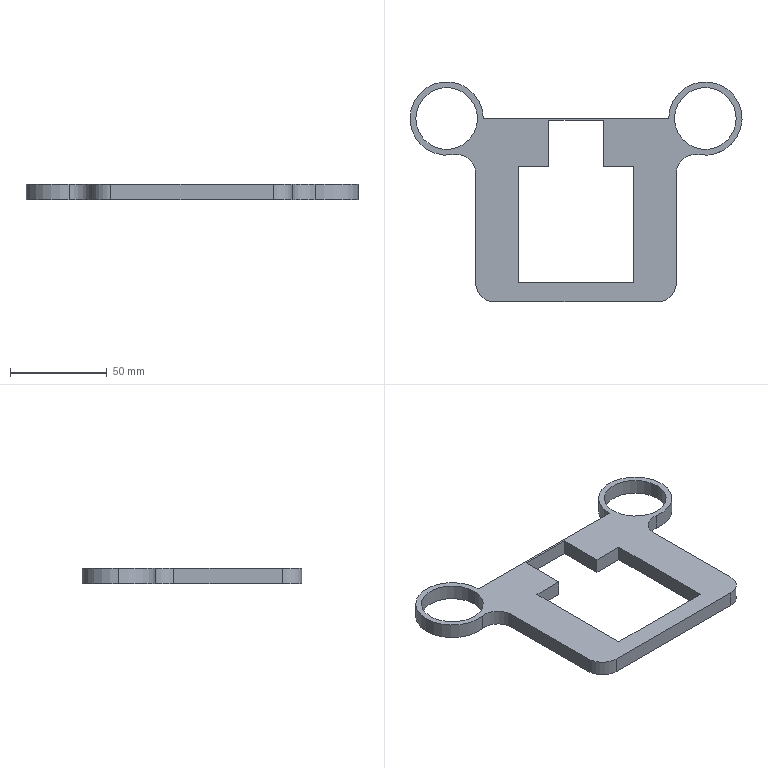Part | SolidWorks | features Extrusion 1 | 1 solid | 25 faces | box 172 x 114 x 8 mm | volume 50080 mm3 | plane 14 | cylinder 11 | commonest cylinder face diameters 20 x4 32 x4 38 x3
STEP:
#1=CARTESIAN_POINT('',(50.608,35.447,8.));
#2=VERTEX_POINT('',#1);
#3=CARTESIAN_POINT('',(82.608,35.447,8.));
#4=VERTEX_POINT('',#3);
#5=CARTESIAN_POINT('',(66.608,35.447,8.));
#6=DIRECTION('',(0.,0.,1.));
#7=DIRECTION('',(1.,0.,0.));
#8=AXIS2_PLACEMENT_3D('',#5,#6,#7);
#9=CIRCLE('',#8,16.);
#10=EDGE_CURVE('',#2,#4,#9,.T.);
#11=ORIENTED_EDGE('',*,*,#10,.T.);
#12=CARTESIAN_POINT('',(82.608,35.447,0.));
#13=VERTEX_POINT('',#12);
#14=CARTESIAN_POINT('',(82.608,35.447,8.));
#15=DIRECTION('',(0.,0.,-1.));
#16=VECTOR('',#15,1000.);
#17=LINE('',#14,#16);
#18=EDGE_CURVE('',#4,#13,#17,.T.);
#19=ORIENTED_EDGE('',*,*,#18,.T.);
#20=CARTESIAN_POINT('',(50.608,35.447,0.));
#21=VERTEX_POINT('',#20);
#22=CARTESIAN_POINT('',(66.608,35.447,0.));
#23=DIRECTION('',(0.,0.,1.));
#24=DIRECTION('',(1.,0.,0.));
#25=AXIS2_PLACEMENT_3D('',#22,#23,#24);
#26=CIRCLE('',#25,16.);
#27=EDGE_CURVE('',#21,#13,#26,.T.);
#28=ORIENTED_EDGE('',*,*,#27,.F.);
#29=CARTESIAN_POINT('',(50.608,35.447,8.));
#30=DIRECTION('',(0.,0.,-1.));
#31=VECTOR('',#30,1000.);
#32=LINE('',#29,#31);
#33=EDGE_CURVE('',#2,#21,#32,.T.);
#34=ORIENTED_EDGE('',*,*,#33,.F.);
#35=EDGE_LOOP('',(#11,#19,#28,#34));
#36=FACE_OUTER_BOUND('',#35,.T.);
#37=CARTESIAN_POINT('',(66.608,35.447,8.));
#38=DIRECTION('',(0.,0.,-1.));
#39=DIRECTION('',(-1.,0.,0.));
#40=AXIS2_PLACEMENT_3D('',#37,#38,#39);
#41=CYLINDRICAL_SURFACE('',#40,16.);
#42=ADVANCED_FACE('',(#36),#41,.F.);
#43=CARTESIAN_POINT('',(-83.392,35.447,8.));
#44=VERTEX_POINT('',#43);
#45=CARTESIAN_POINT('',(-51.392,35.447,8.));
#46=VERTEX_POINT('',#45);
#47=CARTESIAN_POINT('',(-67.392,35.447,8.));
#48=DIRECTION('',(0.,0.,1.));
#49=DIRECTION('',(1.,0.,0.));
#50=AXIS2_PLACEMENT_3D('',#47,#48,#49);
#51=CIRCLE('',#50,16.);
#52=EDGE_CURVE('',#44,#46,#51,.T.);
#53=ORIENTED_EDGE('',*,*,#52,.T.);
#54=CARTESIAN_POINT('',(-51.392,35.447,0.));
#55=VERTEX_POINT('',#54);
#56=CARTESIAN_POINT('',(-51.392,35.447,8.));
#57=DIRECTION('',(0.,0.,-1.));
#58=VECTOR('',#57,1000.);
#59=LINE('',#56,#58);
#60=EDGE_CURVE('',#46,#55,#59,.T.);
#61=ORIENTED_EDGE('',*,*,#60,.T.);
#62=CARTESIAN_POINT('',(-83.392,35.447,0.));
#63=VERTEX_POINT('',#62);
#64=CARTESIAN_POINT('',(-67.392,35.447,0.));
#65=DIRECTION('',(0.,0.,1.));
#66=DIRECTION('',(1.,0.,0.));
#67=AXIS2_PLACEMENT_3D('',#64,#65,#66);
#68=CIRCLE('',#67,16.);
#69=EDGE_CURVE('',#63,#55,#68,.T.);
#70=ORIENTED_EDGE('',*,*,#69,.F.);
#71=CARTESIAN_POINT('',(-83.392,35.447,8.));
#72=DIRECTION('',(0.,0.,-1.));
#73=VECTOR('',#72,1000.);
#74=LINE('',#71,#73);
#75=EDGE_CURVE('',#44,#63,#74,.T.);
#76=ORIENTED_EDGE('',*,*,#75,.F.);
#77=EDGE_LOOP('',(#53,#61,#70,#76));
#78=FACE_OUTER_BOUND('',#77,.T.);
#79=CARTESIAN_POINT('',(-67.392,35.447,8.));
#80=DIRECTION('',(0.,0.,-1.));
#81=DIRECTION('',(-1.,0.,0.));
#82=AXIS2_PLACEMENT_3D('',#79,#80,#81);
#83=CYLINDRICAL_SURFACE('',#82,16.);
#84=ADVANCED_FACE('',(#78),#83,.F.);
#85=CARTESIAN_POINT('',(-86.392,35.447,8.));
#86=VERTEX_POINT('',#85);
#87=CARTESIAN_POINT('',(-64.116,16.731,8.));
#88=VERTEX_POINT('',#87);
#89=CARTESIAN_POINT('',(-67.392,35.447,8.));
#90=DIRECTION('',(0.,0.,1.));
#91=DIRECTION('',(1.,0.,0.));
#92=AXIS2_PLACEMENT_3D('',#89,#90,#91);
#93=CIRCLE('',#92,19.);
#94=EDGE_CURVE('',#86,#88,#93,.T.);
#95=ORIENTED_EDGE('',*,*,#94,.F.);
#96=CARTESIAN_POINT('',(-86.392,35.447,0.));
#97=VERTEX_POINT('',#96);
#98=CARTESIAN_POINT('',(-86.392,35.447,8.));
#99=DIRECTION('',(0.,0.,-1.));
#100=VECTOR('',#99,1000.);
#101=LINE('',#98,#100);
#102=EDGE_CURVE('',#86,#97,#101,.T.);
#103=ORIENTED_EDGE('',*,*,#102,.T.);
#104=CARTESIAN_POINT('',(-64.116,16.731,0.));
#105=VERTEX_POINT('',#104);
#106=CARTESIAN_POINT('',(-67.392,35.447,0.));
#107=DIRECTION('',(0.,0.,1.));
#108=DIRECTION('',(1.,0.,0.));
#109=AXIS2_PLACEMENT_3D('',#106,#107,#108);
#110=CIRCLE('',#109,19.);
#111=EDGE_CURVE('',#97,#105,#110,.T.);
#112=ORIENTED_EDGE('',*,*,#111,.T.);
#113=CARTESIAN_POINT('',(-64.116,16.731,8.));
#114=DIRECTION('',(0.,0.,-1.));
#115=VECTOR('',#114,1000.);
#116=LINE('',#113,#115);
#117=EDGE_CURVE('',#88,#105,#116,.T.);
#118=ORIENTED_EDGE('',*,*,#117,.F.);
#119=EDGE_LOOP('',(#95,#103,#112,#118));
#120=FACE_OUTER_BOUND('',#119,.T.);
#121=CARTESIAN_POINT('',(-67.392,35.447,8.));
#122=DIRECTION('',(0.,0.,-1.));
#123=DIRECTION('',(-1.,0.,0.));
#124=AXIS2_PLACEMENT_3D('',#121,#122,#123);
#125=CYLINDRICAL_SURFACE('',#124,19.);
#126=ADVANCED_FACE('',(#120),#125,.T.);
#127=CARTESIAN_POINT('',(-14.392,34.447,0.));
#128=VERTEX_POINT('',#127);
#129=CARTESIAN_POINT('',(13.608,34.447,0.));
#130=VERTEX_POINT('',#129);
#131=CARTESIAN_POINT('',(0.,34.447,0.));
#132=DIRECTION('',(1.,0.,0.));
#133=VECTOR('',#132,1000.);
#134=LINE('',#131,#133);
#135=EDGE_CURVE('',#128,#130,#134,.T.);
#136=ORIENTED_EDGE('',*,*,#135,.T.);
#137=CARTESIAN_POINT('',(13.608,34.447,8.));
#138=VERTEX_POINT('',#137);
#139=CARTESIAN_POINT('',(13.608,34.447,8.));
#140=DIRECTION('',(0.,0.,-1.));
#141=VECTOR('',#140,1000.);
#142=LINE('',#139,#141);
#143=EDGE_CURVE('',#138,#130,#142,.T.);
#144=ORIENTED_EDGE('',*,*,#143,.F.);
#145=CARTESIAN_POINT('',(-14.392,34.447,8.));
#146=VERTEX_POINT('',#145);
#147=CARTESIAN_POINT('',(0.,34.447,8.));
#148=DIRECTION('',(1.,0.,0.));
#149=VECTOR('',#148,1000.);
#150=LINE('',#147,#149);
#151=EDGE_CURVE('',#146,#138,#150,.T.);
#152=ORIENTED_EDGE('',*,*,#151,.F.);
#153=CARTESIAN_POINT('',(-14.392,34.447,8.));
#154=DIRECTION('',(0.,0.,-1.));
#155=VECTOR('',#154,1000.);
#156=LINE('',#153,#155);
#157=EDGE_CURVE('',#146,#128,#156,.T.);
#158=ORIENTED_EDGE('',*,*,#157,.T.);
#159=EDGE_LOOP('',(#136,#144,#152,#158));
#160=FACE_OUTER_BOUND('',#159,.T.);
#161=CARTESIAN_POINT('',(0.,34.447,8.));
#162=DIRECTION('',(0.,1.,0.));
#163=DIRECTION('',(-1.,0.,0.));
#164=AXIS2_PLACEMENT_3D('',#161,#162,#163);
#165=PLANE('',#164);
#166=ADVANCED_FACE('',(#160),#165,.F.);
#167=CARTESIAN_POINT('',(13.608,10.447,0.));
#168=VERTEX_POINT('',#167);
#169=CARTESIAN_POINT('',(13.608,0.,0.));
#170=DIRECTION('',(0.,-1.,0.));
#171=VECTOR('',#170,1000.);
#172=LINE('',#169,#171);
#173=EDGE_CURVE('',#130,#168,#172,.T.);
#174=ORIENTED_EDGE('',*,*,#173,.T.);
#175=CARTESIAN_POINT('',(13.608,10.447,8.));
#176=VERTEX_POINT('',#175);
#177=CARTESIAN_POINT('',(13.608,10.447,8.));
#178=DIRECTION('',(0.,0.,-1.));
#179=VECTOR('',#178,1000.);
#180=LINE('',#177,#179);
#181=EDGE_CURVE('',#176,#168,#180,.T.);
#182=ORIENTED_EDGE('',*,*,#181,.F.);
#183=CARTESIAN_POINT('',(13.608,0.,8.));
#184=DIRECTION('',(0.,-1.,0.));
#185=VECTOR('',#184,1000.);
#186=LINE('',#183,#185);
#187=EDGE_CURVE('',#138,#176,#186,.T.);
#188=ORIENTED_EDGE('',*,*,#187,.F.);
#189=ORIENTED_EDGE('',*,*,#143,.T.);
#190=EDGE_LOOP('',(#174,#182,#188,#189));
#191=FACE_OUTER_BOUND('',#190,.T.);
#192=CARTESIAN_POINT('',(13.608,0.,8.));
#193=DIRECTION('',(1.,0.,0.));
#194=DIRECTION('',(0.,1.,0.));
#195=AXIS2_PLACEMENT_3D('',#192,#193,#194);
#196=PLANE('',#195);
#197=ADVANCED_FACE('',(#191),#196,.F.);
#198=CARTESIAN_POINT('',(29.608,10.447,0.));
#199=VERTEX_POINT('',#198);
#200=CARTESIAN_POINT('',(0.,10.447,0.));
#201=DIRECTION('',(1.,0.,0.));
#202=VECTOR('',#201,1000.);
#203=LINE('',#200,#202);
#204=EDGE_CURVE('',#168,#199,#203,.T.);
#205=ORIENTED_EDGE('',*,*,#204,.T.);
#206=CARTESIAN_POINT('',(29.608,10.447,8.));
#207=VERTEX_POINT('',#206);
#208=CARTESIAN_POINT('',(29.608,10.447,8.));
#209=DIRECTION('',(0.,0.,-1.));
#210=VECTOR('',#209,1000.);
#211=LINE('',#208,#210);
#212=EDGE_CURVE('',#207,#199,#211,.T.);
#213=ORIENTED_EDGE('',*,*,#212,.F.);
#214=CARTESIAN_POINT('',(0.,10.447,8.));
#215=DIRECTION('',(1.,0.,0.));
#216=VECTOR('',#215,1000.);
#217=LINE('',#214,#216);
#218=EDGE_CURVE('',#176,#207,#217,.T.);
#219=ORIENTED_EDGE('',*,*,#218,.F.);
#220=ORIENTED_EDGE('',*,*,#181,.T.);
#221=EDGE_LOOP('',(#205,#213,#219,#220));
#222=FACE_OUTER_BOUND('',#221,.T.);
#223=CARTESIAN_POINT('',(0.,10.447,8.));
#224=DIRECTION('',(0.,1.,0.));
#225=DIRECTION('',(0.,0.,1.));
#226=AXIS2_PLACEMENT_3D('',#223,#224,#225);
#227=PLANE('',#226);
#228=ADVANCED_FACE('',(#222),#227,.F.);
#229=CARTESIAN_POINT('',(29.608,-49.553,0.));
#230=VERTEX_POINT('',#229);
#231=CARTESIAN_POINT('',(29.608,0.,0.));
#232=DIRECTION('',(0.,-1.,0.));
#233=VECTOR('',#232,1000.);
#234=LINE('',#231,#233);
#235=EDGE_CURVE('',#199,#230,#234,.T.);
#236=ORIENTED_EDGE('',*,*,#235,.T.);
#237=CARTESIAN_POINT('',(29.608,-49.553,8.));
#238=VERTEX_POINT('',#237);
#239=CARTESIAN_POINT('',(29.608,-49.553,8.));
#240=DIRECTION('',(0.,0.,-1.));
#241=VECTOR('',#240,1000.);
#242=LINE('',#239,#241);
#243=EDGE_CURVE('',#238,#230,#242,.T.);
#244=ORIENTED_EDGE('',*,*,#243,.F.);
#245=CARTESIAN_POINT('',(29.608,0.,8.));
#246=DIRECTION('',(0.,-1.,0.));
#247=VECTOR('',#246,1000.);
#248=LINE('',#245,#247);
#249=EDGE_CURVE('',#207,#238,#248,.T.);
#250=ORIENTED_EDGE('',*,*,#249,.F.);
#251=ORIENTED_EDGE('',*,*,#212,.T.);
#252=EDGE_LOOP('',(#236,#244,#250,#251));
#253=FACE_OUTER_BOUND('',#252,.T.);
#254=CARTESIAN_POINT('',(29.608,0.,8.));
#255=DIRECTION('',(1.,0.,0.));
#256=DIRECTION('',(0.,1.,0.));
#257=AXIS2_PLACEMENT_3D('',#254,#255,#256);
#258=PLANE('',#257);
#259=ADVANCED_FACE('',(#253),#258,.F.);
#260=CARTESIAN_POINT('',(-30.392,-49.553,0.));
#261=VERTEX_POINT('',#260);
#262=CARTESIAN_POINT('',(0.,-49.553,0.));
#263=DIRECTION('',(-1.,0.,0.));
#264=VECTOR('',#263,1000.);
#265=LINE('',#262,#264);
#266=EDGE_CURVE('',#230,#261,#265,.T.);
#267=ORIENTED_EDGE('',*,*,#266,.T.);
#268=CARTESIAN_POINT('',(-30.392,-49.553,8.));
#269=VERTEX_POINT('',#268);
#270=CARTESIAN_POINT('',(-30.392,-49.553,8.));
#271=DIRECTION('',(0.,0.,-1.));
#272=VECTOR('',#271,1000.);
#273=LINE('',#270,#272);
#274=EDGE_CURVE('',#269,#261,#273,.T.);
#275=ORIENTED_EDGE('',*,*,#274,.F.);
#276=CARTESIAN_POINT('',(0.,-49.553,8.));
#277=DIRECTION('',(-1.,0.,0.));
#278=VECTOR('',#277,1000.);
#279=LINE('',#276,#278);
#280=EDGE_CURVE('',#238,#269,#279,.T.);
#281=ORIENTED_EDGE('',*,*,#280,.F.);
#282=ORIENTED_EDGE('',*,*,#243,.T.);
#283=EDGE_LOOP('',(#267,#275,#281,#282));
#284=FACE_OUTER_BOUND('',#283,.T.);
#285=CARTESIAN_POINT('',(0.,-49.553,8.));
#286=DIRECTION('',(0.,-1.,0.));
#287=DIRECTION('',(0.,0.,-1.));
#288=AXIS2_PLACEMENT_3D('',#285,#286,#287);
#289=PLANE('',#288);
#290=ADVANCED_FACE('',(#284),#289,.F.);
#291=CARTESIAN_POINT('',(-30.392,10.447,0.));
#292=VERTEX_POINT('',#291);
#293=CARTESIAN_POINT('',(-30.392,0.,0.));
#294=DIRECTION('',(0.,1.,0.));
#295=VECTOR('',#294,1000.);
#296=LINE('',#293,#295);
#297=EDGE_CURVE('',#261,#292,#296,.T.);
#298=ORIENTED_EDGE('',*,*,#297,.T.);
#299=CARTESIAN_POINT('',(-30.392,10.447,8.));
#300=VERTEX_POINT('',#299);
#301=CARTESIAN_POINT('',(-30.392,10.447,8.));
#302=DIRECTION('',(0.,0.,-1.));
#303=VECTOR('',#302,1000.);
#304=LINE('',#301,#303);
#305=EDGE_CURVE('',#300,#292,#304,.T.);
#306=ORIENTED_EDGE('',*,*,#305,.F.);
#307=CARTESIAN_POINT('',(-30.392,0.,8.));
#308=DIRECTION('',(0.,1.,0.));
#309=VECTOR('',#308,1000.);
#310=LINE('',#307,#309);
#311=EDGE_CURVE('',#269,#300,#310,.T.);
#312=ORIENTED_EDGE('',*,*,#311,.F.);
#313=ORIENTED_EDGE('',*,*,#274,.T.);
#314=EDGE_LOOP('',(#298,#306,#312,#313));
#315=FACE_OUTER_BOUND('',#314,.T.);
#316=CARTESIAN_POINT('',(-30.392,0.,8.));
#317=DIRECTION('',(-1.,0.,0.));
#318=DIRECTION('',(0.,-1.,0.));
#319=AXIS2_PLACEMENT_3D('',#316,#317,#318);
#320=PLANE('',#319);
#321=ADVANCED_FACE('',(#315),#320,.F.);
#322=CARTESIAN_POINT('',(-14.392,10.447,0.));
#323=VERTEX_POINT('',#322);
#324=CARTESIAN_POINT('',(0.,10.447,0.));
#325=DIRECTION('',(1.,0.,0.));
#326=VECTOR('',#325,1000.);
#327=LINE('',#324,#326);
#328=EDGE_CURVE('',#292,#323,#327,.T.);
#329=ORIENTED_EDGE('',*,*,#328,.T.);
#330=CARTESIAN_POINT('',(-14.392,10.447,8.));
#331=VERTEX_POINT('',#330);
#332=CARTESIAN_POINT('',(-14.392,10.447,8.));
#333=DIRECTION('',(0.,0.,-1.));
#334=VECTOR('',#333,1000.);
#335=LINE('',#332,#334);
#336=EDGE_CURVE('',#331,#323,#335,.T.);
#337=ORIENTED_EDGE('',*,*,#336,.F.);
#338=CARTESIAN_POINT('',(0.,10.447,8.));
#339=DIRECTION('',(1.,0.,0.));
#340=VECTOR('',#339,1000.);
#341=LINE('',#338,#340);
#342=EDGE_CURVE('',#300,#331,#341,.T.);
#343=ORIENTED_EDGE('',*,*,#342,.F.);
#344=ORIENTED_EDGE('',*,*,#305,.T.);
#345=EDGE_LOOP('',(#329,#337,#343,#344));
#346=FACE_OUTER_BOUND('',#345,.T.);
#347=CARTESIAN_POINT('',(0.,10.447,8.));
#348=DIRECTION('',(0.,1.,0.));
#349=DIRECTION('',(0.,0.,1.));
#350=AXIS2_PLACEMENT_3D('',#347,#348,#349);
#351=PLANE('',#350);
#352=ADVANCED_FACE('',(#346),#351,.F.);
#353=CARTESIAN_POINT('',(63.332,16.731,0.));
#354=VERTEX_POINT('',#353);
#355=CARTESIAN_POINT('',(47.608,35.447,0.));
#356=VERTEX_POINT('',#355);
#357=CARTESIAN_POINT('',(66.608,35.447,0.));
#358=DIRECTION('',(0.,0.,1.));
#359=DIRECTION('',(1.,0.,0.));
#360=AXIS2_PLACEMENT_3D('',#357,#358,#359);
#361=CIRCLE('',#360,19.);
#362=EDGE_CURVE('',#354,#356,#361,.T.);
#363=ORIENTED_EDGE('',*,*,#362,.T.);
#364=CARTESIAN_POINT('',(47.608,35.447,8.));
#365=VERTEX_POINT('',#364);
#366=CARTESIAN_POINT('',(47.608,35.447,8.));
#367=DIRECTION('',(0.,0.,-1.));
#368=VECTOR('',#367,1000.);
#369=LINE('',#366,#368);
#370=EDGE_CURVE('',#365,#356,#369,.T.);
#371=ORIENTED_EDGE('',*,*,#370,.F.);
#372=CARTESIAN_POINT('',(63.332,16.731,8.));
#373=VERTEX_POINT('',#372);
#374=CARTESIAN_POINT('',(66.608,35.447,8.));
#375=DIRECTION('',(0.,0.,1.));
#376=DIRECTION('',(1.,0.,0.));
#377=AXIS2_PLACEMENT_3D('',#374,#375,#376);
#378=CIRCLE('',#377,19.);
#379=EDGE_CURVE('',#373,#365,#378,.T.);
#380=ORIENTED_EDGE('',*,*,#379,.F.);
#381=CARTESIAN_POINT('',(63.332,16.731,8.));
#382=DIRECTION('',(0.,0.,-1.));
#383=VECTOR('',#382,1000.);
#384=LINE('',#381,#383);
#385=EDGE_CURVE('',#373,#354,#384,.T.);
#386=ORIENTED_EDGE('',*,*,#385,.T.);
#387=EDGE_LOOP('',(#363,#371,#380,#386));
#388=FACE_OUTER_BOUND('',#387,.T.);
#389=CARTESIAN_POINT('',(66.608,35.447,8.));
#390=DIRECTION('',(0.,0.,-1.));
#391=DIRECTION('',(-1.,0.,0.));
#392=AXIS2_PLACEMENT_3D('',#389,#390,#391);
#393=CYLINDRICAL_SURFACE('',#392,19.);
#394=ADVANCED_FACE('',(#388),#393,.T.);
#395=CARTESIAN_POINT('',(-48.392,35.447,0.));
#396=VERTEX_POINT('',#395);
#397=CARTESIAN_POINT('',(0.,35.447,0.));
#398=DIRECTION('',(-1.,0.,0.));
#399=VECTOR('',#398,1000.);
#400=LINE('',#397,#399);
#401=EDGE_CURVE('',#356,#396,#400,.T.);
#402=ORIENTED_EDGE('',*,*,#401,.T.);
#403=CARTESIAN_POINT('',(-48.392,35.447,8.));
#404=VERTEX_POINT('',#403);
#405=CARTESIAN_POINT('',(-48.392,35.447,8.));
#406=DIRECTION('',(0.,0.,-1.));
#407=VECTOR('',#406,1000.);
#408=LINE('',#405,#407);
#409=EDGE_CURVE('',#404,#396,#408,.T.);
#410=ORIENTED_EDGE('',*,*,#409,.F.);
#411=CARTESIAN_POINT('',(0.,35.447,8.));
#412=DIRECTION('',(-1.,0.,0.));
#413=VECTOR('',#412,1000.);
#414=LINE('',#411,#413);
#415=EDGE_CURVE('',#365,#404,#414,.T.);
#416=ORIENTED_EDGE('',*,*,#415,.F.);
#417=ORIENTED_EDGE('',*,*,#370,.T.);
#418=EDGE_LOOP('',(#402,#410,#416,#417));
#419=FACE_OUTER_BOUND('',#418,.T.);
#420=CARTESIAN_POINT('',(0.,35.447,8.));
#421=DIRECTION('',(0.,-1.,0.));
#422=DIRECTION('',(0.,0.,-1.));
#423=AXIS2_PLACEMENT_3D('',#420,#421,#422);
#424=PLANE('',#423);
#425=ADVANCED_FACE('',(#419),#424,.F.);
#426=ORIENTED_EDGE('',*,*,#102,.F.);
#427=CARTESIAN_POINT('',(-67.392,35.447,8.));
#428=DIRECTION('',(0.,0.,1.));
#429=DIRECTION('',(1.,0.,0.));
#430=AXIS2_PLACEMENT_3D('',#427,#428,#429);
#431=CIRCLE('',#430,19.);
#432=EDGE_CURVE('',#404,#86,#431,.T.);
#433=ORIENTED_EDGE('',*,*,#432,.F.);
#434=ORIENTED_EDGE('',*,*,#409,.T.);
#435=CARTESIAN_POINT('',(-67.392,35.447,0.));
#436=DIRECTION('',(0.,0.,1.));
#437=DIRECTION('',(1.,0.,0.));
#438=AXIS2_PLACEMENT_3D('',#435,#436,#437);
#439=CIRCLE('',#438,19.);
#440=EDGE_CURVE('',#396,#97,#439,.T.);
#441=ORIENTED_EDGE('',*,*,#440,.T.);
#442=EDGE_LOOP('',(#426,#433,#434,#441));
#443=FACE_OUTER_BOUND('',#442,.T.);
#444=CARTESIAN_POINT('',(-67.392,35.447,8.));
#445=DIRECTION('',(0.,0.,-1.));
#446=DIRECTION('',(-1.,0.,0.));
#447=AXIS2_PLACEMENT_3D('',#444,#445,#446);
#448=CYLINDRICAL_SURFACE('',#447,19.);
#449=ADVANCED_FACE('',(#443),#448,.T.);
#450=CARTESIAN_POINT('',(-52.392,6.881,0.));
#451=VERTEX_POINT('',#450);
#452=CARTESIAN_POINT('',(-62.392,6.881,0.));
#453=DIRECTION('',(0.,0.,1.));
#454=DIRECTION('',(1.,0.,0.));
#455=AXIS2_PLACEMENT_3D('',#452,#453,#454);
#456=CIRCLE('',#455,10.);
#457=EDGE_CURVE('',#451,#105,#456,.T.);
#458=ORIENTED_EDGE('',*,*,#457,.F.);
#459=CARTESIAN_POINT('',(-52.392,6.881,8.));
#460=VERTEX_POINT('',#459);
#461=CARTESIAN_POINT('',(-52.392,6.881,8.));
#462=DIRECTION('',(0.,0.,-1.));
#463=VECTOR('',#462,1000.);
#464=LINE('',#461,#463);
#465=EDGE_CURVE('',#460,#451,#464,.T.);
#466=ORIENTED_EDGE('',*,*,#465,.F.);
#467=CARTESIAN_POINT('',(-62.392,6.881,8.));
#468=DIRECTION('',(0.,0.,1.));
#469=DIRECTION('',(1.,0.,0.));
#470=AXIS2_PLACEMENT_3D('',#467,#468,#469);
#471=CIRCLE('',#470,10.);
#472=EDGE_CURVE('',#460,#88,#471,.T.);
#473=ORIENTED_EDGE('',*,*,#472,.T.);
#474=ORIENTED_EDGE('',*,*,#117,.T.);
#475=EDGE_LOOP('',(#458,#466,#473,#474));
#476=FACE_OUTER_BOUND('',#475,.T.);
#477=CARTESIAN_POINT('',(-62.392,6.881,8.));
#478=DIRECTION('',(0.,0.,-1.));
#479=DIRECTION('',(-1.,0.,0.));
#480=AXIS2_PLACEMENT_3D('',#477,#478,#479);
#481=CYLINDRICAL_SURFACE('',#480,10.);
#482=ADVANCED_FACE('',(#476),#481,.F.);
#483=CARTESIAN_POINT('',(-52.392,-49.553,0.));
#484=VERTEX_POINT('',#483);
#485=CARTESIAN_POINT('',(-52.392,0.,0.));
#486=DIRECTION('',(0.,-1.,0.));
#487=VECTOR('',#486,1000.);
#488=LINE('',#485,#487);
#489=EDGE_CURVE('',#451,#484,#488,.T.);
#490=ORIENTED_EDGE('',*,*,#489,.T.);
#491=CARTESIAN_POINT('',(-52.392,-49.553,8.));
#492=VERTEX_POINT('',#491);
#493=CARTESIAN_POINT('',(-52.392,-49.553,8.));
#494=DIRECTION('',(0.,0.,-1.));
#495=VECTOR('',#494,1000.);
#496=LINE('',#493,#495);
#497=EDGE_CURVE('',#492,#484,#496,.T.);
#498=ORIENTED_EDGE('',*,*,#497,.F.);
#499=CARTESIAN_POINT('',(-52.392,0.,8.));
#500=DIRECTION('',(0.,-1.,0.));
#501=VECTOR('',#500,1000.);
#502=LINE('',#499,#501);
#503=EDGE_CURVE('',#460,#492,#502,.T.);
#504=ORIENTED_EDGE('',*,*,#503,.F.);
#505=ORIENTED_EDGE('',*,*,#465,.T.);
#506=EDGE_LOOP('',(#490,#498,#504,#505));
#507=FACE_OUTER_BOUND('',#506,.T.);
#508=CARTESIAN_POINT('',(-52.392,0.,8.));
#509=DIRECTION('',(1.,0.,0.));
#510=DIRECTION('',(0.,1.,0.));
#511=AXIS2_PLACEMENT_3D('',#508,#509,#510);
#512=PLANE('',#511);
#513=ADVANCED_FACE('',(#507),#512,.F.);
#514=CARTESIAN_POINT('',(-42.392,-59.553,0.));
#515=VERTEX_POINT('',#514);
#516=CARTESIAN_POINT('',(-42.392,-49.553,0.));
#517=DIRECTION('',(0.,0.,1.));
#518=DIRECTION('',(1.,0.,0.));
#519=AXIS2_PLACEMENT_3D('',#516,#517,#518);
#520=CIRCLE('',#519,10.);
#521=EDGE_CURVE('',#484,#515,#520,.T.);
#522=ORIENTED_EDGE('',*,*,#521,.T.);
#523=CARTESIAN_POINT('',(-42.392,-59.553,8.));
#524=VERTEX_POINT('',#523);
#525=CARTESIAN_POINT('',(-42.392,-59.553,8.));
#526=DIRECTION('',(0.,0.,-1.));
#527=VECTOR('',#526,1000.);
#528=LINE('',#525,#527);
#529=EDGE_CURVE('',#524,#515,#528,.T.);
#530=ORIENTED_EDGE('',*,*,#529,.F.);
#531=CARTESIAN_POINT('',(-42.392,-49.553,8.));
#532=DIRECTION('',(0.,0.,1.));
#533=DIRECTION('',(1.,0.,0.));
#534=AXIS2_PLACEMENT_3D('',#531,#532,#533);
#535=CIRCLE('',#534,10.);
#536=EDGE_CURVE('',#492,#524,#535,.T.);
#537=ORIENTED_EDGE('',*,*,#536,.F.);
#538=ORIENTED_EDGE('',*,*,#497,.T.);
#539=EDGE_LOOP('',(#522,#530,#537,#538));
#540=FACE_OUTER_BOUND('',#539,.T.);
#541=CARTESIAN_POINT('',(-42.392,-49.553,8.));
#542=DIRECTION('',(0.,0.,-1.));
#543=DIRECTION('',(-1.,0.,0.));
#544=AXIS2_PLACEMENT_3D('',#541,#542,#543);
#545=CYLINDRICAL_SURFACE('',#544,10.);
#546=ADVANCED_FACE('',(#540),#545,.T.);
#547=CARTESIAN_POINT('',(41.608,-59.553,0.));
#548=VERTEX_POINT('',#547);
#549=CARTESIAN_POINT('',(0.,-59.553,0.));
#550=DIRECTION('',(1.,0.,0.));
#551=VECTOR('',#550,1000.);
#552=LINE('',#549,#551);
#553=EDGE_CURVE('',#515,#548,#552,.T.);
#554=ORIENTED_EDGE('',*,*,#553,.T.);
#555=CARTESIAN_POINT('',(41.608,-59.553,8.));
#556=VERTEX_POINT('',#555);
#557=CARTESIAN_POINT('',(41.608,-59.553,8.));
#558=DIRECTION('',(0.,0.,-1.));
#559=VECTOR('',#558,1000.);
#560=LINE('',#557,#559);
#561=EDGE_CURVE('',#556,#548,#560,.T.);
#562=ORIENTED_EDGE('',*,*,#561,.F.);
#563=CARTESIAN_POINT('',(0.,-59.553,8.));
#564=DIRECTION('',(1.,0.,0.));
#565=VECTOR('',#564,1000.);
#566=LINE('',#563,#565);
#567=EDGE_CURVE('',#524,#556,#566,.T.);
#568=ORIENTED_EDGE('',*,*,#567,.F.);
#569=ORIENTED_EDGE('',*,*,#529,.T.);
#570=EDGE_LOOP('',(#554,#562,#568,#569));
#571=FACE_OUTER_BOUND('',#570,.T.);
#572=CARTESIAN_POINT('',(0.,-59.553,8.));
#573=DIRECTION('',(0.,1.,0.));
#574=DIRECTION('',(0.,0.,1.));
#575=AXIS2_PLACEMENT_3D('',#572,#573,#574);
#576=PLANE('',#575);
#577=ADVANCED_FACE('',(#571),#576,.F.);
#578=CARTESIAN_POINT('',(51.608,-49.553,0.));
#579=VERTEX_POINT('',#578);
#580=CARTESIAN_POINT('',(41.608,-49.553,0.));
#581=DIRECTION('',(0.,0.,-1.));
#582=DIRECTION('',(1.,0.,0.));
#583=AXIS2_PLACEMENT_3D('',#580,#581,#582);
#584=CIRCLE('',#583,10.);
#585=EDGE_CURVE('',#579,#548,#584,.T.);
#586=ORIENTED_EDGE('',*,*,#585,.F.);
#587=CARTESIAN_POINT('',(51.608,-49.553,8.));
#588=VERTEX_POINT('',#587);
#589=CARTESIAN_POINT('',(51.608,-49.553,8.));
#590=DIRECTION('',(0.,0.,-1.));
#591=VECTOR('',#590,1000.);
#592=LINE('',#589,#591);
#593=EDGE_CURVE('',#588,#579,#592,.T.);
#594=ORIENTED_EDGE('',*,*,#593,.F.);
#595=CARTESIAN_POINT('',(41.608,-49.553,8.));
#596=DIRECTION('',(0.,0.,-1.));
#597=DIRECTION('',(1.,0.,0.));
#598=AXIS2_PLACEMENT_3D('',#595,#596,#597);
#599=CIRCLE('',#598,10.);
#600=EDGE_CURVE('',#588,#556,#599,.T.);
#601=ORIENTED_EDGE('',*,*,#600,.T.);
#602=ORIENTED_EDGE('',*,*,#561,.T.);
#603=EDGE_LOOP('',(#586,#594,#601,#602));
#604=FACE_OUTER_BOUND('',#603,.T.);
#605=CARTESIAN_POINT('',(41.608,-49.553,8.));
#606=DIRECTION('',(0.,0.,-1.));
#607=DIRECTION('',(-1.,0.,0.));
#608=AXIS2_PLACEMENT_3D('',#605,#606,#607);
#609=CYLINDRICAL_SURFACE('',#608,10.);
#610=ADVANCED_FACE('',(#604),#609,.T.);
#611=CARTESIAN_POINT('',(51.608,6.881,0.));
#612=VERTEX_POINT('',#611);
#613=CARTESIAN_POINT('',(51.608,0.,0.));
#614=DIRECTION('',(0.,-1.,0.));
#615=VECTOR('',#614,1000.);
#616=LINE('',#613,#615);
#617=EDGE_CURVE('',#612,#579,#616,.T.);
#618=ORIENTED_EDGE('',*,*,#617,.F.);
#619=CARTESIAN_POINT('',(51.608,6.881,8.));
#620=VERTEX_POINT('',#619);
#621=CARTESIAN_POINT('',(51.608,6.881,8.));
#622=DIRECTION('',(0.,0.,-1.));
#623=VECTOR('',#622,1000.);
#624=LINE('',#621,#623);
#625=EDGE_CURVE('',#620,#612,#624,.T.);
#626=ORIENTED_EDGE('',*,*,#625,.F.);
#627=CARTESIAN_POINT('',(51.608,0.,8.));
#628=DIRECTION('',(0.,-1.,0.));
#629=VECTOR('',#628,1000.);
#630=LINE('',#627,#629);
#631=EDGE_CURVE('',#620,#588,#630,.T.);
#632=ORIENTED_EDGE('',*,*,#631,.T.);
#633=ORIENTED_EDGE('',*,*,#593,.T.);
#634=EDGE_LOOP('',(#618,#626,#632,#633));
#635=FACE_OUTER_BOUND('',#634,.T.);
#636=CARTESIAN_POINT('',(51.608,0.,8.));
#637=DIRECTION('',(1.,0.,0.));
#638=DIRECTION('',(0.,1.,0.));
#639=AXIS2_PLACEMENT_3D('',#636,#637,#638);
#640=PLANE('',#639);
#641=ADVANCED_FACE('',(#635),#640,.T.);
#642=ORIENTED_EDGE('',*,*,#60,.F.);
#643=CARTESIAN_POINT('',(-67.392,35.447,8.));
#644=DIRECTION('',(0.,0.,1.));
#645=DIRECTION('',(1.,0.,0.));
#646=AXIS2_PLACEMENT_3D('',#643,#644,#645);
#647=CIRCLE('',#646,16.);
#648=EDGE_CURVE('',#46,#44,#647,.T.);
#649=ORIENTED_EDGE('',*,*,#648,.T.);
#650=ORIENTED_EDGE('',*,*,#75,.T.);
#651=CARTESIAN_POINT('',(-67.392,35.447,0.));
#652=DIRECTION('',(0.,0.,1.));
#653=DIRECTION('',(1.,0.,0.));
#654=AXIS2_PLACEMENT_3D('',#651,#652,#653);
#655=CIRCLE('',#654,16.);
#656=EDGE_CURVE('',#55,#63,#655,.T.);
#657=ORIENTED_EDGE('',*,*,#656,.F.);
#658=EDGE_LOOP('',(#642,#649,#650,#657));
#659=FACE_OUTER_BOUND('',#658,.T.);
#660=CARTESIAN_POINT('',(-67.392,35.447,8.));
#661=DIRECTION('',(0.,0.,-1.));
#662=DIRECTION('',(-1.,0.,0.));
#663=AXIS2_PLACEMENT_3D('',#660,#661,#662);
#664=CYLINDRICAL_SURFACE('',#663,16.);
#665=ADVANCED_FACE('',(#659),#664,.F.);
#666=CARTESIAN_POINT('',(-14.392,0.,0.));
#667=DIRECTION('',(0.,1.,0.));
#668=VECTOR('',#667,1000.);
#669=LINE('',#666,#668);
#670=EDGE_CURVE('',#323,#128,#669,.T.);
#671=ORIENTED_EDGE('',*,*,#670,.T.);
#672=ORIENTED_EDGE('',*,*,#157,.F.);
#673=CARTESIAN_POINT('',(-14.392,0.,8.));
#674=DIRECTION('',(0.,1.,0.));
#675=VECTOR('',#674,1000.);
#676=LINE('',#673,#675);
#677=EDGE_CURVE('',#331,#146,#676,.T.);
#678=ORIENTED_EDGE('',*,*,#677,.F.);
#679=ORIENTED_EDGE('',*,*,#336,.T.);
#680=EDGE_LOOP('',(#671,#672,#678,#679));
#681=FACE_OUTER_BOUND('',#680,.T.);
#682=CARTESIAN_POINT('',(-14.392,0.,8.));
#683=DIRECTION('',(-1.,0.,0.));
#684=DIRECTION('',(0.,0.,1.));
#685=AXIS2_PLACEMENT_3D('',#682,#683,#684);
#686=PLANE('',#685);
#687=ADVANCED_FACE('',(#681),#686,.F.);
#688=CARTESIAN_POINT('',(61.608,6.881,0.));
#689=DIRECTION('',(0.,0.,1.));
#690=DIRECTION('',(1.,0.,0.));
#691=AXIS2_PLACEMENT_3D('',#688,#689,#690);
#692=CIRCLE('',#691,10.);
#693=EDGE_CURVE('',#354,#612,#692,.T.);
#694=ORIENTED_EDGE('',*,*,#693,.F.);
#695=ORIENTED_EDGE('',*,*,#385,.F.);
#696=CARTESIAN_POINT('',(61.608,6.881,8.));
#697=DIRECTION('',(0.,0.,1.));
#698=DIRECTION('',(1.,0.,0.));
#699=AXIS2_PLACEMENT_3D('',#696,#697,#698);
#700=CIRCLE('',#699,10.);
#701=EDGE_CURVE('',#373,#620,#700,.T.);
#702=ORIENTED_EDGE('',*,*,#701,.T.);
#703=ORIENTED_EDGE('',*,*,#625,.T.);
#704=EDGE_LOOP('',(#694,#695,#702,#703));
#705=FACE_OUTER_BOUND('',#704,.T.);
#706=CARTESIAN_POINT('',(61.608,6.881,8.));
#707=DIRECTION('',(0.,0.,-1.));
#708=DIRECTION('',(-1.,0.,0.));
#709=AXIS2_PLACEMENT_3D('',#706,#707,#708);
#710=CYLINDRICAL_SURFACE('',#709,10.);
#711=ADVANCED_FACE('',(#705),#710,.F.);
#712=ORIENTED_EDGE('',*,*,#18,.F.);
#713=CARTESIAN_POINT('',(66.608,35.447,8.));
#714=DIRECTION('',(0.,0.,1.));
#715=DIRECTION('',(1.,0.,0.));
#716=AXIS2_PLACEMENT_3D('',#713,#714,#715);
#717=CIRCLE('',#716,16.);
#718=EDGE_CURVE('',#4,#2,#717,.T.);
#719=ORIENTED_EDGE('',*,*,#718,.T.);
#720=ORIENTED_EDGE('',*,*,#33,.T.);
#721=CARTESIAN_POINT('',(66.608,35.447,0.));
#722=DIRECTION('',(0.,0.,1.));
#723=DIRECTION('',(1.,0.,0.));
#724=AXIS2_PLACEMENT_3D('',#721,#722,#723);
#725=CIRCLE('',#724,16.);
#726=EDGE_CURVE('',#13,#21,#725,.T.);
#727=ORIENTED_EDGE('',*,*,#726,.F.);
#728=EDGE_LOOP('',(#712,#719,#720,#727));
#729=FACE_OUTER_BOUND('',#728,.T.);
#730=CARTESIAN_POINT('',(66.608,35.447,8.));
#731=DIRECTION('',(0.,0.,-1.));
#732=DIRECTION('',(-1.,0.,0.));
#733=AXIS2_PLACEMENT_3D('',#730,#731,#732);
#734=CYLINDRICAL_SURFACE('',#733,16.);
#735=ADVANCED_FACE('',(#729),#734,.F.);
#736=ORIENTED_EDGE('',*,*,#379,.T.);
#737=ORIENTED_EDGE('',*,*,#415,.T.);
#738=ORIENTED_EDGE('',*,*,#432,.T.);
#739=ORIENTED_EDGE('',*,*,#94,.T.);
#740=ORIENTED_EDGE('',*,*,#472,.F.);
#741=ORIENTED_EDGE('',*,*,#503,.T.);
#742=ORIENTED_EDGE('',*,*,#536,.T.);
#743=ORIENTED_EDGE('',*,*,#567,.T.);
#744=ORIENTED_EDGE('',*,*,#600,.F.);
#745=ORIENTED_EDGE('',*,*,#631,.F.);
#746=ORIENTED_EDGE('',*,*,#701,.F.);
#747=EDGE_LOOP('',(#736,#737,#738,#739,#740,#741,#742,#743,#744,#745,#746));
#748=FACE_OUTER_BOUND('',#747,.T.);
#749=ORIENTED_EDGE('',*,*,#151,.T.);
#750=ORIENTED_EDGE('',*,*,#187,.T.);
#751=ORIENTED_EDGE('',*,*,#218,.T.);
#752=ORIENTED_EDGE('',*,*,#249,.T.);
#753=ORIENTED_EDGE('',*,*,#280,.T.);
#754=ORIENTED_EDGE('',*,*,#311,.T.);
#755=ORIENTED_EDGE('',*,*,#342,.T.);
#756=ORIENTED_EDGE('',*,*,#677,.T.);
#757=EDGE_LOOP('',(#749,#750,#751,#752,#753,#754,#755,#756));
#758=FACE_BOUND('',#757,.T.);
#759=ORIENTED_EDGE('',*,*,#52,.F.);
#760=ORIENTED_EDGE('',*,*,#648,.F.);
#761=EDGE_LOOP('',(#759,#760));
#762=FACE_BOUND('',#761,.T.);
#763=ORIENTED_EDGE('',*,*,#10,.F.);
#764=ORIENTED_EDGE('',*,*,#718,.F.);
#765=EDGE_LOOP('',(#763,#764));
#766=FACE_BOUND('',#765,.T.);
#767=CARTESIAN_POINT('',(0.,0.,8.));
#768=DIRECTION('',(0.,0.,1.));
#769=DIRECTION('',(1.,0.,0.));
#770=AXIS2_PLACEMENT_3D('',#767,#768,#769);
#771=PLANE('',#770);
#772=ADVANCED_FACE('',(#748,#758,#762,#766),#771,.T.);
#773=ORIENTED_EDGE('',*,*,#362,.F.);
#774=ORIENTED_EDGE('',*,*,#693,.T.);
#775=ORIENTED_EDGE('',*,*,#617,.T.);
#776=ORIENTED_EDGE('',*,*,#585,.T.);
#777=ORIENTED_EDGE('',*,*,#553,.F.);
#778=ORIENTED_EDGE('',*,*,#521,.F.);
#779=ORIENTED_EDGE('',*,*,#489,.F.);
#780=ORIENTED_EDGE('',*,*,#457,.T.);
#781=ORIENTED_EDGE('',*,*,#111,.F.);
#782=ORIENTED_EDGE('',*,*,#440,.F.);
#783=ORIENTED_EDGE('',*,*,#401,.F.);
#784=EDGE_LOOP('',(#773,#774,#775,#776,#777,#778,#779,#780,#781,#782,#783));
#785=FACE_OUTER_BOUND('',#784,.T.);
#786=ORIENTED_EDGE('',*,*,#135,.F.);
#787=ORIENTED_EDGE('',*,*,#670,.F.);
#788=ORIENTED_EDGE('',*,*,#328,.F.);
#789=ORIENTED_EDGE('',*,*,#297,.F.);
#790=ORIENTED_EDGE('',*,*,#266,.F.);
#791=ORIENTED_EDGE('',*,*,#235,.F.);
#792=ORIENTED_EDGE('',*,*,#204,.F.);
#793=ORIENTED_EDGE('',*,*,#173,.F.);
#794=EDGE_LOOP('',(#786,#787,#788,#789,#790,#791,#792,#793));
#795=FACE_BOUND('',#794,.T.);
#796=ORIENTED_EDGE('',*,*,#69,.T.);
#797=ORIENTED_EDGE('',*,*,#656,.T.);
#798=EDGE_LOOP('',(#796,#797));
#799=FACE_BOUND('',#798,.T.);
#800=ORIENTED_EDGE('',*,*,#27,.T.);
#801=ORIENTED_EDGE('',*,*,#726,.T.);
#802=EDGE_LOOP('',(#800,#801));
#803=FACE_BOUND('',#802,.T.);
#804=CARTESIAN_POINT('',(0.,0.,0.));
#805=DIRECTION('',(0.,0.,1.));
#806=DIRECTION('',(1.,0.,0.));
#807=AXIS2_PLACEMENT_3D('',#804,#805,#806);
#808=PLANE('',#807);
#809=ADVANCED_FACE('',(#785,#795,#799,#803),#808,.F.);
#810=CLOSED_SHELL('',(#42,#84,#126,#166,#197,#228,#259,#290,#321,#352,#394,#425,#449,#482,#513,#546,#577,#610,#641,#665,#687,#711,#735,#772,#809));
#811=MANIFOLD_SOLID_BREP('',#810);
#812=CARTESIAN_POINT('',(0.,0.,0.));
#813=DIRECTION('',(0.,0.,1.));
#814=DIRECTION('',(1.,0.,0.));
#815=AXIS2_PLACEMENT_3D('',#812,#813,#814);
#816=(LENGTH_UNIT()NAMED_UNIT(*)SI_UNIT(.MILLI.,.METRE.));
#817=UNCERTAINTY_MEASURE_WITH_UNIT(LENGTH_MEASURE(0.00001),#816,'','');
#818=(NAMED_UNIT(*)PLANE_ANGLE_UNIT()SI_UNIT($,.RADIAN.));
#819=(NAMED_UNIT(*)SI_UNIT($,.STERADIAN.)SOLID_ANGLE_UNIT());
#820=(GEOMETRIC_REPRESENTATION_CONTEXT(3)GLOBAL_UNCERTAINTY_ASSIGNED_CONTEXT((#817))GLOBAL_UNIT_ASSIGNED_CONTEXT((#816,#818,#819))REPRESENTATION_CONTEXT('',''));
#821=ADVANCED_BREP_SHAPE_REPRESENTATION('',(#811,#815),#820);